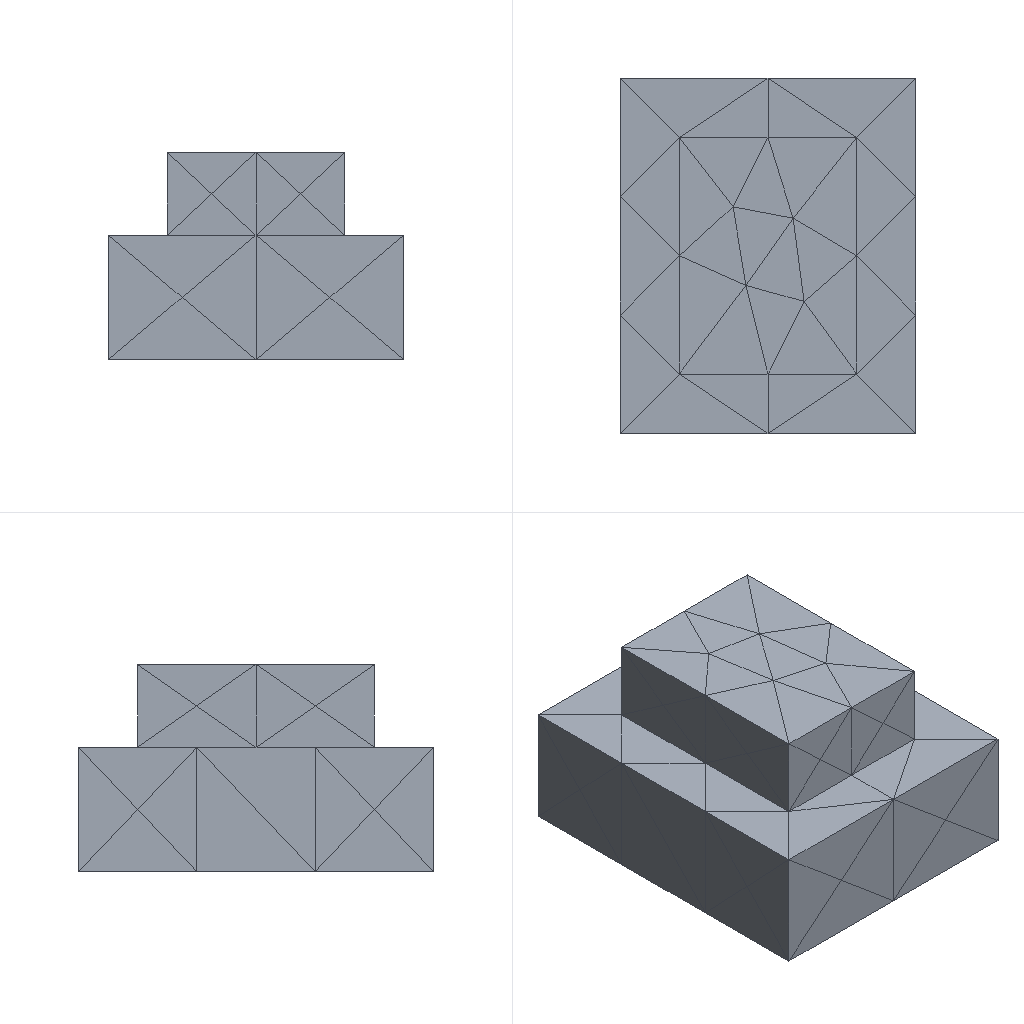Simulation study | ansys mapdl
Set-up summary:
category,name,step,type,value,unit,region
solver,ansys_mapdl
units,mm-N-s-tonne (MPa),,inferred,E=210000 density=
analysis,model,,static
mesh,nodes,,,465
mesh,elements,,,238
element_type,SOLID187,,,238
material,mat 1,,E,210000
material,mat 1,,nu,0.3
load,,model,body load temp,,,all
load,,model,force,"1000 [dir=(0, 0, -1) n=99]",,node list
bc,,model,fixed,"[dofs=UX,UY,UZ n=560]",,node list
Ansys APDL input file, long lists of numbers shortened:
/COM,ANSYS RELEASE 2026 R1           BUILD 26.1      UP20260202       09:10:49
/PREP7
/NOPR
/TITLE,2
ANTYPE, 0
*IF,_CDRDOFF,EQ,1,THEN     !if solid model was read in
_CDRDOFF=             !reset flag, numoffs already performed
*ELSE              !offset database for the following FE model
NUMOFF,NODE,      465
NUMOFF,ELEM,      238
NUMOFF,MAT ,        1
NUMOFF,TYPE,        1
*ENDIF
*SET,_RETURN ,  0.
*SET,_STATUS ,  0.
*SET,_UIQR   ,  99.
*SET,__FLOATPARAMETER__,  465.
DOF,DELETE
ETBLOCK,        1,        1
(2i9,19a9)
        1      187        0        0        0        0        0        0        0        0        0        0        0        0        0        0        0        0        0        0        0
       -1
NBLOCK,6,SOLID,       465,       465
(3i9,6e21.13e3)
        1        0        0 4.3000000000000E+001-1.2000000000000E+001 8.4000000000000E+000
! (464 more lines like these left out)
N,UNBL,LOC,       -1,
EBLOCK,19,SOLID,       238,       238
(19i10)
         1         1         1         1         0         0         0         0        10         0         1       267         8        10        35       280         9       281       282
! (475 more lines like these left out)
        -1
MPTEMP,UNBL, 1, 1,  0.    ,
MPDATA,UNBL, 1,EX  ,       1, 1,  210000.000    ,
MPTEMP,UNBL, 1, 1,  0.    ,
MPDATA,UNBL, 1,NUXY,       1, 1, 0.3    ,
MPTEMP,UNBL, 1, 1,  0.    ,
MPDATA,UNBL, 1,PRXY,       1, 1, 0.3    ,
EXTOPT,ATTR,      0,      0,      0
EXTOPT,ESIZE,  0,  0.
EXTOPT,ACLEAR,      0
TREF,  0.
IRLF,  0
BFUNIF,TEMP,_TINY
ACEL,  0.    ,  0.    ,  0.
OMEGA,  0.    ,  0.    ,  0.
DOMEGA,  0.    ,  0.    ,  0.
CGLOC,  0.    ,  0.    ,  0.
CGOMEGA,  0.    ,  0.    ,  0.
DCGOMG,  0.    ,  0.    ,  0.
KUSE,     0
TIME,  0.
ALPHAD,  0.
BETAD,  0.
DMPRAT,  0.
DMPSTR,  0.
CRPLIM, 0.1    ,   0
CRPLIM,  0.    ,   1
NCNV,     0, 1.000000000E+12,     0,  0.    ,  0.
NEQIT,     0
ERESX,DEFA
DBLOCK,       560
(i9,a6,2(pg16.9))
        1  UX    0.00000000      0.00000000
! (559 more lines like these left out)
       -1
FBLOCK,        99
(i9,a6,2(pg16.9))
      182  FZ   -10.1010101      0.00000000
! (98 more lines like these left out)
       -1
/GO
FINISH
Results summary:
result,analysis_type_db,,,static,unstated
result,n_sets,,,1,unstated
result,load_steps[0].set,load_step=1,,1,unstated
result,load_steps[0].substep,load_step=1,,1,unstated
result,load_steps[0].time,load_step=1,,1,unstated
result,load_steps[0].freq,load_step=1,,1,unstated
result,load_steps[0].max_usum,load_step=1,,0.0003834,unstated
result,load_steps[0].max_seqv,load_step=1,,9.444,unstated
result,load_steps[0].reaction_sum.FX,load_step=1,,-7.3328e-12,unstated
result,load_steps[0].reaction_sum.FY,load_step=1,,-7.91545e-12,unstated
result,load_steps[0].reaction_sum.FZ,load_step=1,,1000,unstated
result,load_steps[0].reaction_sum.MX,load_step=1,,0,unstated
result,load_steps[0].reaction_sum.MY,load_step=1,,0,unstated
result,load_steps[0].reaction_sum.MZ,load_step=1,,0,unstated
result,convergence,,,results present for all listed sets,unstated